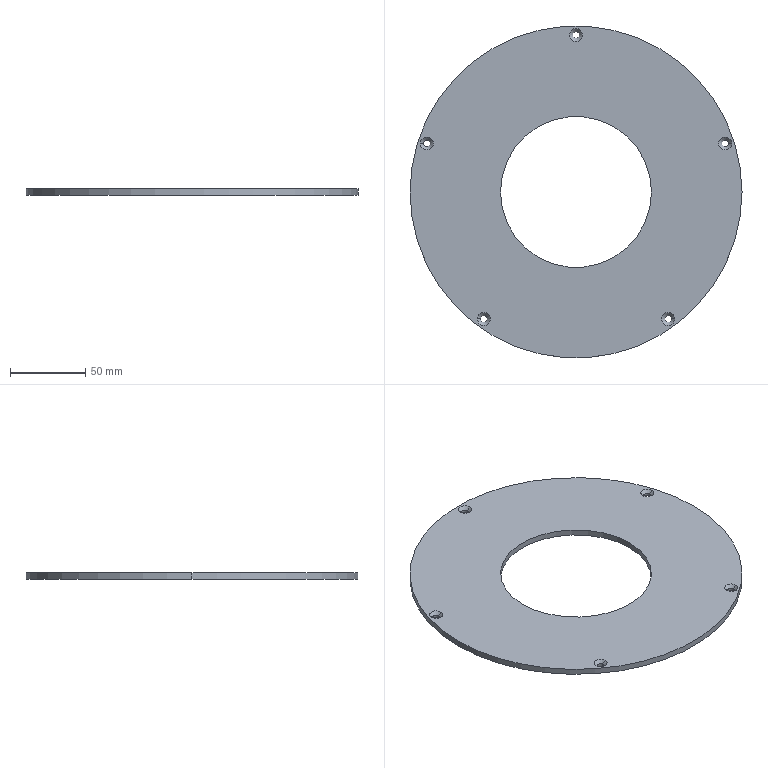Part | SolidWorks | features Extrusion 1, HoleWzd 1 | 1 solid | 26 faces | box 220 x 220 x 4 mm | volume 120125 mm3 | cylinder 14 | cone 10 | plane 2 | commonest cylinder face diameters 4.5 x10 100 x2 220 x2
STEP:
#1=CARTESIAN_POINT('',(-2.25,104.,1.95));
#2=VERTEX_POINT('',#1);
#3=CARTESIAN_POINT('',(2.25,104.,1.95));
#4=VERTEX_POINT('',#3);
#5=CARTESIAN_POINT('',(0.,104.,1.95));
#6=DIRECTION('',(0.,0.,1.));
#7=DIRECTION('',(1.,0.,0.));
#8=AXIS2_PLACEMENT_3D('',#5,#6,#7);
#9=CIRCLE('',#8,2.25);
#10=EDGE_CURVE('',#2,#4,#9,.T.);
#11=ORIENTED_EDGE('',*,*,#10,.F.);
#12=CARTESIAN_POINT('',(-4.3,104.,4.));
#13=VERTEX_POINT('',#12);
#14=CARTESIAN_POINT('',(-4.3,104.,4.));
#15=DIRECTION('',(-0.7071,0.,0.7071));
#16=VECTOR('',#15,1000.);
#17=LINE('',#14,#16);
#18=EDGE_CURVE('',#2,#13,#17,.T.);
#19=ORIENTED_EDGE('',*,*,#18,.T.);
#20=CARTESIAN_POINT('',(4.3,104.,4.));
#21=VERTEX_POINT('',#20);
#22=CARTESIAN_POINT('',(0.,104.,4.));
#23=DIRECTION('',(0.,0.,1.));
#24=DIRECTION('',(1.,0.,0.));
#25=AXIS2_PLACEMENT_3D('',#22,#23,#24);
#26=CIRCLE('',#25,4.3);
#27=EDGE_CURVE('',#13,#21,#26,.T.);
#28=ORIENTED_EDGE('',*,*,#27,.T.);
#29=CARTESIAN_POINT('',(4.3,104.,4.));
#30=DIRECTION('',(0.7071,0.,0.7071));
#31=VECTOR('',#30,1000.);
#32=LINE('',#29,#31);
#33=EDGE_CURVE('',#4,#21,#32,.T.);
#34=ORIENTED_EDGE('',*,*,#33,.F.);
#35=EDGE_LOOP('',(#11,#19,#28,#34));
#36=FACE_OUTER_BOUND('',#35,.T.);
#37=CARTESIAN_POINT('',(0.,104.,4.));
#38=DIRECTION('',(0.,0.,1.));
#39=DIRECTION('',(1.,0.,0.));
#40=AXIS2_PLACEMENT_3D('',#37,#38,#39);
#41=CONICAL_SURFACE('',#40,4.3,0.7854);
#42=ADVANCED_FACE('',(#36),#41,.F.);
#43=CARTESIAN_POINT('',(-2.25,104.,0.));
#44=VERTEX_POINT('',#43);
#45=CARTESIAN_POINT('',(2.25,104.,0.));
#46=VERTEX_POINT('',#45);
#47=CARTESIAN_POINT('',(0.,104.,0.));
#48=DIRECTION('',(0.,0.,1.));
#49=DIRECTION('',(1.,0.,0.));
#50=AXIS2_PLACEMENT_3D('',#47,#48,#49);
#51=CIRCLE('',#50,2.25);
#52=EDGE_CURVE('',#44,#46,#51,.T.);
#53=ORIENTED_EDGE('',*,*,#52,.F.);
#54=CARTESIAN_POINT('',(-2.25,104.,4.));
#55=DIRECTION('',(0.,0.,1.));
#56=VECTOR('',#55,1000.);
#57=LINE('',#54,#56);
#58=EDGE_CURVE('',#44,#2,#57,.T.);
#59=ORIENTED_EDGE('',*,*,#58,.T.);
#60=ORIENTED_EDGE('',*,*,#10,.T.);
#61=CARTESIAN_POINT('',(2.25,104.,4.));
#62=DIRECTION('',(0.,0.,1.));
#63=VECTOR('',#62,1000.);
#64=LINE('',#61,#63);
#65=EDGE_CURVE('',#46,#4,#64,.T.);
#66=ORIENTED_EDGE('',*,*,#65,.F.);
#67=EDGE_LOOP('',(#53,#59,#60,#66));
#68=FACE_OUTER_BOUND('',#67,.T.);
#69=CARTESIAN_POINT('',(0.,104.,4.));
#70=DIRECTION('',(0.,0.,1.));
#71=DIRECTION('',(1.,0.,0.));
#72=AXIS2_PLACEMENT_3D('',#69,#70,#71);
#73=CYLINDRICAL_SURFACE('',#72,2.25);
#74=ADVANCED_FACE('',(#68),#73,.F.);
#75=CARTESIAN_POINT('',(96.66,32.138,1.95));
#76=VERTEX_POINT('',#75);
#77=CARTESIAN_POINT('',(101.16,32.138,1.95));
#78=VERTEX_POINT('',#77);
#79=CARTESIAN_POINT('',(98.91,32.138,1.95));
#80=DIRECTION('',(0.,0.,1.));
#81=DIRECTION('',(1.,0.,0.));
#82=AXIS2_PLACEMENT_3D('',#79,#80,#81);
#83=CIRCLE('',#82,2.25);
#84=EDGE_CURVE('',#76,#78,#83,.T.);
#85=ORIENTED_EDGE('',*,*,#84,.F.);
#86=CARTESIAN_POINT('',(94.61,32.138,4.));
#87=VERTEX_POINT('',#86);
#88=CARTESIAN_POINT('',(94.61,32.138,4.));
#89=DIRECTION('',(-0.7071,0.,0.7071));
#90=VECTOR('',#89,1000.);
#91=LINE('',#88,#90);
#92=EDGE_CURVE('',#76,#87,#91,.T.);
#93=ORIENTED_EDGE('',*,*,#92,.T.);
#94=CARTESIAN_POINT('',(103.21,32.138,4.));
#95=VERTEX_POINT('',#94);
#96=CARTESIAN_POINT('',(98.91,32.138,4.));
#97=DIRECTION('',(0.,0.,1.));
#98=DIRECTION('',(1.,0.,0.));
#99=AXIS2_PLACEMENT_3D('',#96,#97,#98);
#100=CIRCLE('',#99,4.3);
#101=EDGE_CURVE('',#87,#95,#100,.T.);
#102=ORIENTED_EDGE('',*,*,#101,.T.);
#103=CARTESIAN_POINT('',(103.21,32.138,4.));
#104=DIRECTION('',(0.7071,0.,0.7071));
#105=VECTOR('',#104,1000.);
#106=LINE('',#103,#105);
#107=EDGE_CURVE('',#78,#95,#106,.T.);
#108=ORIENTED_EDGE('',*,*,#107,.F.);
#109=EDGE_LOOP('',(#85,#93,#102,#108));
#110=FACE_OUTER_BOUND('',#109,.T.);
#111=CARTESIAN_POINT('',(98.91,32.138,4.));
#112=DIRECTION('',(0.,0.,1.));
#113=DIRECTION('',(1.,0.,0.));
#114=AXIS2_PLACEMENT_3D('',#111,#112,#113);
#115=CONICAL_SURFACE('',#114,4.3,0.7854);
#116=ADVANCED_FACE('',(#110),#115,.F.);
#117=CARTESIAN_POINT('',(96.66,32.138,0.));
#118=VERTEX_POINT('',#117);
#119=CARTESIAN_POINT('',(101.16,32.138,0.));
#120=VERTEX_POINT('',#119);
#121=CARTESIAN_POINT('',(98.91,32.138,0.));
#122=DIRECTION('',(0.,0.,1.));
#123=DIRECTION('',(1.,0.,0.));
#124=AXIS2_PLACEMENT_3D('',#121,#122,#123);
#125=CIRCLE('',#124,2.25);
#126=EDGE_CURVE('',#118,#120,#125,.T.);
#127=ORIENTED_EDGE('',*,*,#126,.F.);
#128=CARTESIAN_POINT('',(96.66,32.138,4.));
#129=DIRECTION('',(0.,0.,1.));
#130=VECTOR('',#129,1000.);
#131=LINE('',#128,#130);
#132=EDGE_CURVE('',#118,#76,#131,.T.);
#133=ORIENTED_EDGE('',*,*,#132,.T.);
#134=ORIENTED_EDGE('',*,*,#84,.T.);
#135=CARTESIAN_POINT('',(101.16,32.138,4.));
#136=DIRECTION('',(0.,0.,1.));
#137=VECTOR('',#136,1000.);
#138=LINE('',#135,#137);
#139=EDGE_CURVE('',#120,#78,#138,.T.);
#140=ORIENTED_EDGE('',*,*,#139,.F.);
#141=EDGE_LOOP('',(#127,#133,#134,#140));
#142=FACE_OUTER_BOUND('',#141,.T.);
#143=CARTESIAN_POINT('',(98.91,32.138,4.));
#144=DIRECTION('',(0.,0.,1.));
#145=DIRECTION('',(1.,0.,0.));
#146=AXIS2_PLACEMENT_3D('',#143,#144,#145);
#147=CYLINDRICAL_SURFACE('',#146,2.25);
#148=ADVANCED_FACE('',(#142),#147,.F.);
#149=CARTESIAN_POINT('',(58.88,-84.138,1.95));
#150=VERTEX_POINT('',#149);
#151=CARTESIAN_POINT('',(63.38,-84.138,1.95));
#152=VERTEX_POINT('',#151);
#153=CARTESIAN_POINT('',(61.13,-84.138,1.95));
#154=DIRECTION('',(0.,0.,1.));
#155=DIRECTION('',(1.,0.,0.));
#156=AXIS2_PLACEMENT_3D('',#153,#154,#155);
#157=CIRCLE('',#156,2.25);
#158=EDGE_CURVE('',#150,#152,#157,.T.);
#159=ORIENTED_EDGE('',*,*,#158,.F.);
#160=CARTESIAN_POINT('',(56.83,-84.138,4.));
#161=VERTEX_POINT('',#160);
#162=CARTESIAN_POINT('',(56.83,-84.138,4.));
#163=DIRECTION('',(-0.7071,0.,0.7071));
#164=VECTOR('',#163,1000.);
#165=LINE('',#162,#164);
#166=EDGE_CURVE('',#150,#161,#165,.T.);
#167=ORIENTED_EDGE('',*,*,#166,.T.);
#168=CARTESIAN_POINT('',(65.43,-84.138,4.));
#169=VERTEX_POINT('',#168);
#170=CARTESIAN_POINT('',(61.13,-84.138,4.));
#171=DIRECTION('',(0.,0.,1.));
#172=DIRECTION('',(1.,0.,0.));
#173=AXIS2_PLACEMENT_3D('',#170,#171,#172);
#174=CIRCLE('',#173,4.3);
#175=EDGE_CURVE('',#161,#169,#174,.T.);
#176=ORIENTED_EDGE('',*,*,#175,.T.);
#177=CARTESIAN_POINT('',(65.43,-84.138,4.));
#178=DIRECTION('',(0.7071,0.,0.7071));
#179=VECTOR('',#178,1000.);
#180=LINE('',#177,#179);
#181=EDGE_CURVE('',#152,#169,#180,.T.);
#182=ORIENTED_EDGE('',*,*,#181,.F.);
#183=EDGE_LOOP('',(#159,#167,#176,#182));
#184=FACE_OUTER_BOUND('',#183,.T.);
#185=CARTESIAN_POINT('',(61.13,-84.138,4.));
#186=DIRECTION('',(0.,0.,1.));
#187=DIRECTION('',(1.,0.,0.));
#188=AXIS2_PLACEMENT_3D('',#185,#186,#187);
#189=CONICAL_SURFACE('',#188,4.3,0.7854);
#190=ADVANCED_FACE('',(#184),#189,.F.);
#191=CARTESIAN_POINT('',(58.88,-84.138,0.));
#192=VERTEX_POINT('',#191);
#193=CARTESIAN_POINT('',(63.38,-84.138,0.));
#194=VERTEX_POINT('',#193);
#195=CARTESIAN_POINT('',(61.13,-84.138,0.));
#196=DIRECTION('',(0.,0.,1.));
#197=DIRECTION('',(1.,0.,0.));
#198=AXIS2_PLACEMENT_3D('',#195,#196,#197);
#199=CIRCLE('',#198,2.25);
#200=EDGE_CURVE('',#192,#194,#199,.T.);
#201=ORIENTED_EDGE('',*,*,#200,.F.);
#202=CARTESIAN_POINT('',(58.88,-84.138,4.));
#203=DIRECTION('',(0.,0.,1.));
#204=VECTOR('',#203,1000.);
#205=LINE('',#202,#204);
#206=EDGE_CURVE('',#192,#150,#205,.T.);
#207=ORIENTED_EDGE('',*,*,#206,.T.);
#208=ORIENTED_EDGE('',*,*,#158,.T.);
#209=CARTESIAN_POINT('',(63.38,-84.138,4.));
#210=DIRECTION('',(0.,0.,1.));
#211=VECTOR('',#210,1000.);
#212=LINE('',#209,#211);
#213=EDGE_CURVE('',#194,#152,#212,.T.);
#214=ORIENTED_EDGE('',*,*,#213,.F.);
#215=EDGE_LOOP('',(#201,#207,#208,#214));
#216=FACE_OUTER_BOUND('',#215,.T.);
#217=CARTESIAN_POINT('',(61.13,-84.138,4.));
#218=DIRECTION('',(0.,0.,1.));
#219=DIRECTION('',(1.,0.,0.));
#220=AXIS2_PLACEMENT_3D('',#217,#218,#219);
#221=CYLINDRICAL_SURFACE('',#220,2.25);
#222=ADVANCED_FACE('',(#216),#221,.F.);
#223=CARTESIAN_POINT('',(-63.38,-84.138,1.95));
#224=VERTEX_POINT('',#223);
#225=CARTESIAN_POINT('',(-58.88,-84.138,1.95));
#226=VERTEX_POINT('',#225);
#227=CARTESIAN_POINT('',(-61.13,-84.138,1.95));
#228=DIRECTION('',(0.,0.,1.));
#229=DIRECTION('',(1.,0.,0.));
#230=AXIS2_PLACEMENT_3D('',#227,#228,#229);
#231=CIRCLE('',#230,2.25);
#232=EDGE_CURVE('',#224,#226,#231,.T.);
#233=ORIENTED_EDGE('',*,*,#232,.F.);
#234=CARTESIAN_POINT('',(-65.43,-84.138,4.));
#235=VERTEX_POINT('',#234);
#236=CARTESIAN_POINT('',(-65.43,-84.138,4.));
#237=DIRECTION('',(-0.7071,0.,0.7071));
#238=VECTOR('',#237,1000.);
#239=LINE('',#236,#238);
#240=EDGE_CURVE('',#224,#235,#239,.T.);
#241=ORIENTED_EDGE('',*,*,#240,.T.);
#242=CARTESIAN_POINT('',(-56.83,-84.138,4.));
#243=VERTEX_POINT('',#242);
#244=CARTESIAN_POINT('',(-61.13,-84.138,4.));
#245=DIRECTION('',(0.,0.,1.));
#246=DIRECTION('',(1.,0.,0.));
#247=AXIS2_PLACEMENT_3D('',#244,#245,#246);
#248=CIRCLE('',#247,4.3);
#249=EDGE_CURVE('',#235,#243,#248,.T.);
#250=ORIENTED_EDGE('',*,*,#249,.T.);
#251=CARTESIAN_POINT('',(-56.83,-84.138,4.));
#252=DIRECTION('',(0.7071,0.,0.7071));
#253=VECTOR('',#252,1000.);
#254=LINE('',#251,#253);
#255=EDGE_CURVE('',#226,#243,#254,.T.);
#256=ORIENTED_EDGE('',*,*,#255,.F.);
#257=EDGE_LOOP('',(#233,#241,#250,#256));
#258=FACE_OUTER_BOUND('',#257,.T.);
#259=CARTESIAN_POINT('',(-61.13,-84.138,4.));
#260=DIRECTION('',(0.,0.,1.));
#261=DIRECTION('',(1.,0.,0.));
#262=AXIS2_PLACEMENT_3D('',#259,#260,#261);
#263=CONICAL_SURFACE('',#262,4.3,0.7854);
#264=ADVANCED_FACE('',(#258),#263,.F.);
#265=CARTESIAN_POINT('',(-63.38,-84.138,0.));
#266=VERTEX_POINT('',#265);
#267=CARTESIAN_POINT('',(-58.88,-84.138,0.));
#268=VERTEX_POINT('',#267);
#269=CARTESIAN_POINT('',(-61.13,-84.138,0.));
#270=DIRECTION('',(0.,0.,1.));
#271=DIRECTION('',(1.,0.,0.));
#272=AXIS2_PLACEMENT_3D('',#269,#270,#271);
#273=CIRCLE('',#272,2.25);
#274=EDGE_CURVE('',#266,#268,#273,.T.);
#275=ORIENTED_EDGE('',*,*,#274,.F.);
#276=CARTESIAN_POINT('',(-63.38,-84.138,4.));
#277=DIRECTION('',(0.,0.,1.));
#278=VECTOR('',#277,1000.);
#279=LINE('',#276,#278);
#280=EDGE_CURVE('',#266,#224,#279,.T.);
#281=ORIENTED_EDGE('',*,*,#280,.T.);
#282=ORIENTED_EDGE('',*,*,#232,.T.);
#283=CARTESIAN_POINT('',(-58.88,-84.138,4.));
#284=DIRECTION('',(0.,0.,1.));
#285=VECTOR('',#284,1000.);
#286=LINE('',#283,#285);
#287=EDGE_CURVE('',#268,#226,#286,.T.);
#288=ORIENTED_EDGE('',*,*,#287,.F.);
#289=EDGE_LOOP('',(#275,#281,#282,#288));
#290=FACE_OUTER_BOUND('',#289,.T.);
#291=CARTESIAN_POINT('',(-61.13,-84.138,4.));
#292=DIRECTION('',(0.,0.,1.));
#293=DIRECTION('',(1.,0.,0.));
#294=AXIS2_PLACEMENT_3D('',#291,#292,#293);
#295=CYLINDRICAL_SURFACE('',#294,2.25);
#296=ADVANCED_FACE('',(#290),#295,.F.);
#297=CARTESIAN_POINT('',(-101.16,32.138,1.95));
#298=VERTEX_POINT('',#297);
#299=CARTESIAN_POINT('',(-96.66,32.138,1.95));
#300=VERTEX_POINT('',#299);
#301=CARTESIAN_POINT('',(-98.91,32.138,1.95));
#302=DIRECTION('',(0.,0.,1.));
#303=DIRECTION('',(1.,0.,0.));
#304=AXIS2_PLACEMENT_3D('',#301,#302,#303);
#305=CIRCLE('',#304,2.25);
#306=EDGE_CURVE('',#298,#300,#305,.T.);
#307=ORIENTED_EDGE('',*,*,#306,.F.);
#308=CARTESIAN_POINT('',(-103.21,32.138,4.));
#309=VERTEX_POINT('',#308);
#310=CARTESIAN_POINT('',(-103.21,32.138,4.));
#311=DIRECTION('',(-0.7071,0.,0.7071));
#312=VECTOR('',#311,1000.);
#313=LINE('',#310,#312);
#314=EDGE_CURVE('',#298,#309,#313,.T.);
#315=ORIENTED_EDGE('',*,*,#314,.T.);
#316=CARTESIAN_POINT('',(-94.61,32.138,4.));
#317=VERTEX_POINT('',#316);
#318=CARTESIAN_POINT('',(-98.91,32.138,4.));
#319=DIRECTION('',(0.,0.,1.));
#320=DIRECTION('',(1.,0.,0.));
#321=AXIS2_PLACEMENT_3D('',#318,#319,#320);
#322=CIRCLE('',#321,4.3);
#323=EDGE_CURVE('',#309,#317,#322,.T.);
#324=ORIENTED_EDGE('',*,*,#323,.T.);
#325=CARTESIAN_POINT('',(-94.61,32.138,4.));
#326=DIRECTION('',(0.7071,0.,0.7071));
#327=VECTOR('',#326,1000.);
#328=LINE('',#325,#327);
#329=EDGE_CURVE('',#300,#317,#328,.T.);
#330=ORIENTED_EDGE('',*,*,#329,.F.);
#331=EDGE_LOOP('',(#307,#315,#324,#330));
#332=FACE_OUTER_BOUND('',#331,.T.);
#333=CARTESIAN_POINT('',(-98.91,32.138,4.));
#334=DIRECTION('',(0.,0.,1.));
#335=DIRECTION('',(1.,0.,0.));
#336=AXIS2_PLACEMENT_3D('',#333,#334,#335);
#337=CONICAL_SURFACE('',#336,4.3,0.7854);
#338=ADVANCED_FACE('',(#332),#337,.F.);
#339=CARTESIAN_POINT('',(-101.16,32.138,0.));
#340=VERTEX_POINT('',#339);
#341=CARTESIAN_POINT('',(-96.66,32.138,0.));
#342=VERTEX_POINT('',#341);
#343=CARTESIAN_POINT('',(-98.91,32.138,0.));
#344=DIRECTION('',(0.,0.,1.));
#345=DIRECTION('',(1.,0.,0.));
#346=AXIS2_PLACEMENT_3D('',#343,#344,#345);
#347=CIRCLE('',#346,2.25);
#348=EDGE_CURVE('',#340,#342,#347,.T.);
#349=ORIENTED_EDGE('',*,*,#348,.F.);
#350=CARTESIAN_POINT('',(-101.16,32.138,4.));
#351=DIRECTION('',(0.,0.,1.));
#352=VECTOR('',#351,1000.);
#353=LINE('',#350,#352);
#354=EDGE_CURVE('',#340,#298,#353,.T.);
#355=ORIENTED_EDGE('',*,*,#354,.T.);
#356=ORIENTED_EDGE('',*,*,#306,.T.);
#357=CARTESIAN_POINT('',(-96.66,32.138,4.));
#358=DIRECTION('',(0.,0.,1.));
#359=VECTOR('',#358,1000.);
#360=LINE('',#357,#359);
#361=EDGE_CURVE('',#342,#300,#360,.T.);
#362=ORIENTED_EDGE('',*,*,#361,.F.);
#363=EDGE_LOOP('',(#349,#355,#356,#362));
#364=FACE_OUTER_BOUND('',#363,.T.);
#365=CARTESIAN_POINT('',(-98.91,32.138,4.));
#366=DIRECTION('',(0.,0.,1.));
#367=DIRECTION('',(1.,0.,0.));
#368=AXIS2_PLACEMENT_3D('',#365,#366,#367);
#369=CYLINDRICAL_SURFACE('',#368,2.25);
#370=ADVANCED_FACE('',(#364),#369,.F.);
#371=CARTESIAN_POINT('',(-50.,0.,4.));
#372=VERTEX_POINT('',#371);
#373=CARTESIAN_POINT('',(50.,0.,4.));
#374=VERTEX_POINT('',#373);
#375=CARTESIAN_POINT('',(0.,0.,4.));
#376=DIRECTION('',(0.,0.,1.));
#377=DIRECTION('',(1.,0.,0.));
#378=AXIS2_PLACEMENT_3D('',#375,#376,#377);
#379=CIRCLE('',#378,50.);
#380=EDGE_CURVE('',#372,#374,#379,.T.);
#381=ORIENTED_EDGE('',*,*,#380,.T.);
#382=CARTESIAN_POINT('',(50.,0.,0.));
#383=VERTEX_POINT('',#382);
#384=CARTESIAN_POINT('',(50.,0.,4.));
#385=DIRECTION('',(0.,0.,-1.));
#386=VECTOR('',#385,1000.);
#387=LINE('',#384,#386);
#388=EDGE_CURVE('',#374,#383,#387,.T.);
#389=ORIENTED_EDGE('',*,*,#388,.T.);
#390=CARTESIAN_POINT('',(-50.,0.,0.));
#391=VERTEX_POINT('',#390);
#392=CARTESIAN_POINT('',(0.,0.,0.));
#393=DIRECTION('',(0.,0.,1.));
#394=DIRECTION('',(1.,0.,0.));
#395=AXIS2_PLACEMENT_3D('',#392,#393,#394);
#396=CIRCLE('',#395,50.);
#397=EDGE_CURVE('',#391,#383,#396,.T.);
#398=ORIENTED_EDGE('',*,*,#397,.F.);
#399=CARTESIAN_POINT('',(-50.,0.,4.));
#400=DIRECTION('',(0.,0.,-1.));
#401=VECTOR('',#400,1000.);
#402=LINE('',#399,#401);
#403=EDGE_CURVE('',#372,#391,#402,.T.);
#404=ORIENTED_EDGE('',*,*,#403,.F.);
#405=EDGE_LOOP('',(#381,#389,#398,#404));
#406=FACE_OUTER_BOUND('',#405,.T.);
#407=CARTESIAN_POINT('',(0.,0.,4.));
#408=DIRECTION('',(0.,0.,-1.));
#409=DIRECTION('',(-1.,0.,0.));
#410=AXIS2_PLACEMENT_3D('',#407,#408,#409);
#411=CYLINDRICAL_SURFACE('',#410,50.);
#412=ADVANCED_FACE('',(#406),#411,.F.);
#413=CARTESIAN_POINT('',(110.,0.,4.));
#414=VERTEX_POINT('',#413);
#415=CARTESIAN_POINT('',(-110.,0.,4.));
#416=VERTEX_POINT('',#415);
#417=CARTESIAN_POINT('',(0.,0.,4.));
#418=DIRECTION('',(0.,0.,1.));
#419=DIRECTION('',(1.,0.,0.));
#420=AXIS2_PLACEMENT_3D('',#417,#418,#419);
#421=CIRCLE('',#420,110.);
#422=EDGE_CURVE('',#414,#416,#421,.T.);
#423=ORIENTED_EDGE('',*,*,#422,.F.);
#424=CARTESIAN_POINT('',(110.,0.,0.));
#425=VERTEX_POINT('',#424);
#426=CARTESIAN_POINT('',(110.,0.,4.));
#427=DIRECTION('',(0.,0.,-1.));
#428=VECTOR('',#427,1000.);
#429=LINE('',#426,#428);
#430=EDGE_CURVE('',#414,#425,#429,.T.);
#431=ORIENTED_EDGE('',*,*,#430,.T.);
#432=CARTESIAN_POINT('',(-110.,0.,0.));
#433=VERTEX_POINT('',#432);
#434=CARTESIAN_POINT('',(0.,0.,0.));
#435=DIRECTION('',(0.,0.,1.));
#436=DIRECTION('',(1.,0.,0.));
#437=AXIS2_PLACEMENT_3D('',#434,#435,#436);
#438=CIRCLE('',#437,110.);
#439=EDGE_CURVE('',#425,#433,#438,.T.);
#440=ORIENTED_EDGE('',*,*,#439,.T.);
#441=CARTESIAN_POINT('',(-110.,0.,4.));
#442=DIRECTION('',(0.,0.,-1.));
#443=VECTOR('',#442,1000.);
#444=LINE('',#441,#443);
#445=EDGE_CURVE('',#416,#433,#444,.T.);
#446=ORIENTED_EDGE('',*,*,#445,.F.);
#447=EDGE_LOOP('',(#423,#431,#440,#446));
#448=FACE_OUTER_BOUND('',#447,.T.);
#449=CARTESIAN_POINT('',(0.,0.,4.));
#450=DIRECTION('',(0.,0.,-1.));
#451=DIRECTION('',(-1.,0.,0.));
#452=AXIS2_PLACEMENT_3D('',#449,#450,#451);
#453=CYLINDRICAL_SURFACE('',#452,110.);
#454=ADVANCED_FACE('',(#448),#453,.T.);
#455=CARTESIAN_POINT('',(0.,104.,4.));
#456=DIRECTION('',(0.,0.,1.));
#457=DIRECTION('',(1.,0.,0.));
#458=AXIS2_PLACEMENT_3D('',#455,#456,#457);
#459=CIRCLE('',#458,4.3);
#460=EDGE_CURVE('',#21,#13,#459,.T.);
#461=ORIENTED_EDGE('',*,*,#460,.F.);
#462=ORIENTED_EDGE('',*,*,#27,.F.);
#463=EDGE_LOOP('',(#461,#462));
#464=FACE_BOUND('',#463,.T.);
#465=CARTESIAN_POINT('',(98.91,32.138,4.));
#466=DIRECTION('',(0.,0.,1.));
#467=DIRECTION('',(1.,0.,0.));
#468=AXIS2_PLACEMENT_3D('',#465,#466,#467);
#469=CIRCLE('',#468,4.3);
#470=EDGE_CURVE('',#95,#87,#469,.T.);
#471=ORIENTED_EDGE('',*,*,#470,.F.);
#472=ORIENTED_EDGE('',*,*,#101,.F.);
#473=EDGE_LOOP('',(#471,#472));
#474=FACE_BOUND('',#473,.T.);
#475=CARTESIAN_POINT('',(61.13,-84.138,4.));
#476=DIRECTION('',(0.,0.,1.));
#477=DIRECTION('',(1.,0.,0.));
#478=AXIS2_PLACEMENT_3D('',#475,#476,#477);
#479=CIRCLE('',#478,4.3);
#480=EDGE_CURVE('',#169,#161,#479,.T.);
#481=ORIENTED_EDGE('',*,*,#480,.F.);
#482=ORIENTED_EDGE('',*,*,#175,.F.);
#483=EDGE_LOOP('',(#481,#482));
#484=FACE_BOUND('',#483,.T.);
#485=CARTESIAN_POINT('',(-61.13,-84.138,4.));
#486=DIRECTION('',(0.,0.,1.));
#487=DIRECTION('',(1.,0.,0.));
#488=AXIS2_PLACEMENT_3D('',#485,#486,#487);
#489=CIRCLE('',#488,4.3);
#490=EDGE_CURVE('',#243,#235,#489,.T.);
#491=ORIENTED_EDGE('',*,*,#490,.F.);
#492=ORIENTED_EDGE('',*,*,#249,.F.);
#493=EDGE_LOOP('',(#491,#492));
#494=FACE_BOUND('',#493,.T.);
#495=CARTESIAN_POINT('',(-98.91,32.138,4.));
#496=DIRECTION('',(0.,0.,1.));
#497=DIRECTION('',(1.,0.,0.));
#498=AXIS2_PLACEMENT_3D('',#495,#496,#497);
#499=CIRCLE('',#498,4.3);
#500=EDGE_CURVE('',#317,#309,#499,.T.);
#501=ORIENTED_EDGE('',*,*,#500,.F.);
#502=ORIENTED_EDGE('',*,*,#323,.F.);
#503=EDGE_LOOP('',(#501,#502));
#504=FACE_BOUND('',#503,.T.);
#505=CARTESIAN_POINT('',(0.,0.,4.));
#506=DIRECTION('',(0.,0.,1.));
#507=DIRECTION('',(1.,0.,0.));
#508=AXIS2_PLACEMENT_3D('',#505,#506,#507);
#509=CIRCLE('',#508,110.);
#510=EDGE_CURVE('',#416,#414,#509,.T.);
#511=ORIENTED_EDGE('',*,*,#510,.T.);
#512=ORIENTED_EDGE('',*,*,#422,.T.);
#513=EDGE_LOOP('',(#511,#512));
#514=FACE_OUTER_BOUND('',#513,.T.);
#515=ORIENTED_EDGE('',*,*,#380,.F.);
#516=CARTESIAN_POINT('',(0.,0.,4.));
#517=DIRECTION('',(0.,0.,1.));
#518=DIRECTION('',(1.,0.,0.));
#519=AXIS2_PLACEMENT_3D('',#516,#517,#518);
#520=CIRCLE('',#519,50.);
#521=EDGE_CURVE('',#374,#372,#520,.T.);
#522=ORIENTED_EDGE('',*,*,#521,.F.);
#523=EDGE_LOOP('',(#515,#522));
#524=FACE_BOUND('',#523,.T.);
#525=CARTESIAN_POINT('',(0.,0.,4.));
#526=DIRECTION('',(0.,0.,1.));
#527=DIRECTION('',(1.,0.,0.));
#528=AXIS2_PLACEMENT_3D('',#525,#526,#527);
#529=PLANE('',#528);
#530=ADVANCED_FACE('',(#464,#474,#484,#494,#504,#514,#524),#529,.T.);
#531=CARTESIAN_POINT('',(0.,104.,0.));
#532=DIRECTION('',(0.,0.,1.));
#533=DIRECTION('',(1.,0.,0.));
#534=AXIS2_PLACEMENT_3D('',#531,#532,#533);
#535=CIRCLE('',#534,2.25);
#536=EDGE_CURVE('',#46,#44,#535,.T.);
#537=ORIENTED_EDGE('',*,*,#536,.T.);
#538=ORIENTED_EDGE('',*,*,#52,.T.);
#539=EDGE_LOOP('',(#537,#538));
#540=FACE_BOUND('',#539,.T.);
#541=CARTESIAN_POINT('',(98.91,32.138,0.));
#542=DIRECTION('',(0.,0.,1.));
#543=DIRECTION('',(1.,0.,0.));
#544=AXIS2_PLACEMENT_3D('',#541,#542,#543);
#545=CIRCLE('',#544,2.25);
#546=EDGE_CURVE('',#120,#118,#545,.T.);
#547=ORIENTED_EDGE('',*,*,#546,.T.);
#548=ORIENTED_EDGE('',*,*,#126,.T.);
#549=EDGE_LOOP('',(#547,#548));
#550=FACE_BOUND('',#549,.T.);
#551=CARTESIAN_POINT('',(61.13,-84.138,0.));
#552=DIRECTION('',(0.,0.,1.));
#553=DIRECTION('',(1.,0.,0.));
#554=AXIS2_PLACEMENT_3D('',#551,#552,#553);
#555=CIRCLE('',#554,2.25);
#556=EDGE_CURVE('',#194,#192,#555,.T.);
#557=ORIENTED_EDGE('',*,*,#556,.T.);
#558=ORIENTED_EDGE('',*,*,#200,.T.);
#559=EDGE_LOOP('',(#557,#558));
#560=FACE_BOUND('',#559,.T.);
#561=CARTESIAN_POINT('',(-61.13,-84.138,0.));
#562=DIRECTION('',(0.,0.,1.));
#563=DIRECTION('',(1.,0.,0.));
#564=AXIS2_PLACEMENT_3D('',#561,#562,#563);
#565=CIRCLE('',#564,2.25);
#566=EDGE_CURVE('',#268,#266,#565,.T.);
#567=ORIENTED_EDGE('',*,*,#566,.T.);
#568=ORIENTED_EDGE('',*,*,#274,.T.);
#569=EDGE_LOOP('',(#567,#568));
#570=FACE_BOUND('',#569,.T.);
#571=CARTESIAN_POINT('',(-98.91,32.138,0.));
#572=DIRECTION('',(0.,0.,1.));
#573=DIRECTION('',(1.,0.,0.));
#574=AXIS2_PLACEMENT_3D('',#571,#572,#573);
#575=CIRCLE('',#574,2.25);
#576=EDGE_CURVE('',#342,#340,#575,.T.);
#577=ORIENTED_EDGE('',*,*,#576,.T.);
#578=ORIENTED_EDGE('',*,*,#348,.T.);
#579=EDGE_LOOP('',(#577,#578));
#580=FACE_BOUND('',#579,.T.);
#581=CARTESIAN_POINT('',(0.,0.,0.));
#582=DIRECTION('',(0.,0.,1.));
#583=DIRECTION('',(1.,0.,0.));
#584=AXIS2_PLACEMENT_3D('',#581,#582,#583);
#585=CIRCLE('',#584,110.);
#586=EDGE_CURVE('',#433,#425,#585,.T.);
#587=ORIENTED_EDGE('',*,*,#586,.F.);
#588=ORIENTED_EDGE('',*,*,#439,.F.);
#589=EDGE_LOOP('',(#587,#588));
#590=FACE_OUTER_BOUND('',#589,.T.);
#591=ORIENTED_EDGE('',*,*,#397,.T.);
#592=CARTESIAN_POINT('',(0.,0.,0.));
#593=DIRECTION('',(0.,0.,1.));
#594=DIRECTION('',(1.,0.,0.));
#595=AXIS2_PLACEMENT_3D('',#592,#593,#594);
#596=CIRCLE('',#595,50.);
#597=EDGE_CURVE('',#383,#391,#596,.T.);
#598=ORIENTED_EDGE('',*,*,#597,.T.);
#599=EDGE_LOOP('',(#591,#598));
#600=FACE_BOUND('',#599,.T.);
#601=CARTESIAN_POINT('',(0.,0.,0.));
#602=DIRECTION('',(0.,0.,1.));
#603=DIRECTION('',(1.,0.,0.));
#604=AXIS2_PLACEMENT_3D('',#601,#602,#603);
#605=PLANE('',#604);
#606=ADVANCED_FACE('',(#540,#550,#560,#570,#580,#590,#600),#605,.F.);
#607=ORIENTED_EDGE('',*,*,#430,.F.);
#608=ORIENTED_EDGE('',*,*,#510,.F.);
#609=ORIENTED_EDGE('',*,*,#445,.T.);
#610=ORIENTED_EDGE('',*,*,#586,.T.);
#611=EDGE_LOOP('',(#607,#608,#609,#610));
#612=FACE_OUTER_BOUND('',#611,.T.);
#613=CARTESIAN_POINT('',(0.,0.,4.));
#614=DIRECTION('',(0.,0.,-1.));
#615=DIRECTION('',(-1.,0.,0.));
#616=AXIS2_PLACEMENT_3D('',#613,#614,#615);
#617=CYLINDRICAL_SURFACE('',#616,110.);
#618=ADVANCED_FACE('',(#612),#617,.T.);
#619=ORIENTED_EDGE('',*,*,#388,.F.);
#620=ORIENTED_EDGE('',*,*,#521,.T.);
#621=ORIENTED_EDGE('',*,*,#403,.T.);
#622=ORIENTED_EDGE('',*,*,#597,.F.);
#623=EDGE_LOOP('',(#619,#620,#621,#622));
#624=FACE_OUTER_BOUND('',#623,.T.);
#625=CARTESIAN_POINT('',(0.,0.,4.));
#626=DIRECTION('',(0.,0.,-1.));
#627=DIRECTION('',(-1.,0.,0.));
#628=AXIS2_PLACEMENT_3D('',#625,#626,#627);
#629=CYLINDRICAL_SURFACE('',#628,50.);
#630=ADVANCED_FACE('',(#624),#629,.F.);
#631=ORIENTED_EDGE('',*,*,#354,.F.);
#632=ORIENTED_EDGE('',*,*,#576,.F.);
#633=ORIENTED_EDGE('',*,*,#361,.T.);
#634=CARTESIAN_POINT('',(-98.91,32.138,1.95));
#635=DIRECTION('',(0.,0.,1.));
#636=DIRECTION('',(1.,0.,0.));
#637=AXIS2_PLACEMENT_3D('',#634,#635,#636);
#638=CIRCLE('',#637,2.25);
#639=EDGE_CURVE('',#300,#298,#638,.T.);
#640=ORIENTED_EDGE('',*,*,#639,.T.);
#641=EDGE_LOOP('',(#631,#632,#633,#640));
#642=FACE_OUTER_BOUND('',#641,.T.);
#643=CARTESIAN_POINT('',(-98.91,32.138,4.));
#644=DIRECTION('',(0.,0.,1.));
#645=DIRECTION('',(1.,0.,0.));
#646=AXIS2_PLACEMENT_3D('',#643,#644,#645);
#647=CYLINDRICAL_SURFACE('',#646,2.25);
#648=ADVANCED_FACE('',(#642),#647,.F.);
#649=ORIENTED_EDGE('',*,*,#314,.F.);
#650=ORIENTED_EDGE('',*,*,#639,.F.);
#651=ORIENTED_EDGE('',*,*,#329,.T.);
#652=ORIENTED_EDGE('',*,*,#500,.T.);
#653=EDGE_LOOP('',(#649,#650,#651,#652));
#654=FACE_OUTER_BOUND('',#653,.T.);
#655=CARTESIAN_POINT('',(-98.91,32.138,4.));
#656=DIRECTION('',(0.,0.,1.));
#657=DIRECTION('',(1.,0.,0.));
#658=AXIS2_PLACEMENT_3D('',#655,#656,#657);
#659=CONICAL_SURFACE('',#658,4.3,0.7854);
#660=ADVANCED_FACE('',(#654),#659,.F.);
#661=ORIENTED_EDGE('',*,*,#280,.F.);
#662=ORIENTED_EDGE('',*,*,#566,.F.);
#663=ORIENTED_EDGE('',*,*,#287,.T.);
#664=CARTESIAN_POINT('',(-61.13,-84.138,1.95));
#665=DIRECTION('',(0.,0.,1.));
#666=DIRECTION('',(1.,0.,0.));
#667=AXIS2_PLACEMENT_3D('',#664,#665,#666);
#668=CIRCLE('',#667,2.25);
#669=EDGE_CURVE('',#226,#224,#668,.T.);
#670=ORIENTED_EDGE('',*,*,#669,.T.);
#671=EDGE_LOOP('',(#661,#662,#663,#670));
#672=FACE_OUTER_BOUND('',#671,.T.);
#673=CARTESIAN_POINT('',(-61.13,-84.138,4.));
#674=DIRECTION('',(0.,0.,1.));
#675=DIRECTION('',(1.,0.,0.));
#676=AXIS2_PLACEMENT_3D('',#673,#674,#675);
#677=CYLINDRICAL_SURFACE('',#676,2.25);
#678=ADVANCED_FACE('',(#672),#677,.F.);
#679=ORIENTED_EDGE('',*,*,#240,.F.);
#680=ORIENTED_EDGE('',*,*,#669,.F.);
#681=ORIENTED_EDGE('',*,*,#255,.T.);
#682=ORIENTED_EDGE('',*,*,#490,.T.);
#683=EDGE_LOOP('',(#679,#680,#681,#682));
#684=FACE_OUTER_BOUND('',#683,.T.);
#685=CARTESIAN_POINT('',(-61.13,-84.138,4.));
#686=DIRECTION('',(0.,0.,1.));
#687=DIRECTION('',(1.,0.,0.));
#688=AXIS2_PLACEMENT_3D('',#685,#686,#687);
#689=CONICAL_SURFACE('',#688,4.3,0.7854);
#690=ADVANCED_FACE('',(#684),#689,.F.);
#691=ORIENTED_EDGE('',*,*,#206,.F.);
#692=ORIENTED_EDGE('',*,*,#556,.F.);
#693=ORIENTED_EDGE('',*,*,#213,.T.);
#694=CARTESIAN_POINT('',(61.13,-84.138,1.95));
#695=DIRECTION('',(0.,0.,1.));
#696=DIRECTION('',(1.,0.,0.));
#697=AXIS2_PLACEMENT_3D('',#694,#695,#696);
#698=CIRCLE('',#697,2.25);
#699=EDGE_CURVE('',#152,#150,#698,.T.);
#700=ORIENTED_EDGE('',*,*,#699,.T.);
#701=EDGE_LOOP('',(#691,#692,#693,#700));
#702=FACE_OUTER_BOUND('',#701,.T.);
#703=CARTESIAN_POINT('',(61.13,-84.138,4.));
#704=DIRECTION('',(0.,0.,1.));
#705=DIRECTION('',(1.,0.,0.));
#706=AXIS2_PLACEMENT_3D('',#703,#704,#705);
#707=CYLINDRICAL_SURFACE('',#706,2.25);
#708=ADVANCED_FACE('',(#702),#707,.F.);
#709=ORIENTED_EDGE('',*,*,#166,.F.);
#710=ORIENTED_EDGE('',*,*,#699,.F.);
#711=ORIENTED_EDGE('',*,*,#181,.T.);
#712=ORIENTED_EDGE('',*,*,#480,.T.);
#713=EDGE_LOOP('',(#709,#710,#711,#712));
#714=FACE_OUTER_BOUND('',#713,.T.);
#715=CARTESIAN_POINT('',(61.13,-84.138,4.));
#716=DIRECTION('',(0.,0.,1.));
#717=DIRECTION('',(1.,0.,0.));
#718=AXIS2_PLACEMENT_3D('',#715,#716,#717);
#719=CONICAL_SURFACE('',#718,4.3,0.7854);
#720=ADVANCED_FACE('',(#714),#719,.F.);
#721=ORIENTED_EDGE('',*,*,#132,.F.);
#722=ORIENTED_EDGE('',*,*,#546,.F.);
#723=ORIENTED_EDGE('',*,*,#139,.T.);
#724=CARTESIAN_POINT('',(98.91,32.138,1.95));
#725=DIRECTION('',(0.,0.,1.));
#726=DIRECTION('',(1.,0.,0.));
#727=AXIS2_PLACEMENT_3D('',#724,#725,#726);
#728=CIRCLE('',#727,2.25);
#729=EDGE_CURVE('',#78,#76,#728,.T.);
#730=ORIENTED_EDGE('',*,*,#729,.T.);
#731=EDGE_LOOP('',(#721,#722,#723,#730));
#732=FACE_OUTER_BOUND('',#731,.T.);
#733=CARTESIAN_POINT('',(98.91,32.138,4.));
#734=DIRECTION('',(0.,0.,1.));
#735=DIRECTION('',(1.,0.,0.));
#736=AXIS2_PLACEMENT_3D('',#733,#734,#735);
#737=CYLINDRICAL_SURFACE('',#736,2.25);
#738=ADVANCED_FACE('',(#732),#737,.F.);
#739=ORIENTED_EDGE('',*,*,#92,.F.);
#740=ORIENTED_EDGE('',*,*,#729,.F.);
#741=ORIENTED_EDGE('',*,*,#107,.T.);
#742=ORIENTED_EDGE('',*,*,#470,.T.);
#743=EDGE_LOOP('',(#739,#740,#741,#742));
#744=FACE_OUTER_BOUND('',#743,.T.);
#745=CARTESIAN_POINT('',(98.91,32.138,4.));
#746=DIRECTION('',(0.,0.,1.));
#747=DIRECTION('',(1.,0.,0.));
#748=AXIS2_PLACEMENT_3D('',#745,#746,#747);
#749=CONICAL_SURFACE('',#748,4.3,0.7854);
#750=ADVANCED_FACE('',(#744),#749,.F.);
#751=ORIENTED_EDGE('',*,*,#58,.F.);
#752=ORIENTED_EDGE('',*,*,#536,.F.);
#753=ORIENTED_EDGE('',*,*,#65,.T.);
#754=CARTESIAN_POINT('',(0.,104.,1.95));
#755=DIRECTION('',(0.,0.,1.));
#756=DIRECTION('',(1.,0.,0.));
#757=AXIS2_PLACEMENT_3D('',#754,#755,#756);
#758=CIRCLE('',#757,2.25);
#759=EDGE_CURVE('',#4,#2,#758,.T.);
#760=ORIENTED_EDGE('',*,*,#759,.T.);
#761=EDGE_LOOP('',(#751,#752,#753,#760));
#762=FACE_OUTER_BOUND('',#761,.T.);
#763=CARTESIAN_POINT('',(0.,104.,4.));
#764=DIRECTION('',(0.,0.,1.));
#765=DIRECTION('',(1.,0.,0.));
#766=AXIS2_PLACEMENT_3D('',#763,#764,#765);
#767=CYLINDRICAL_SURFACE('',#766,2.25);
#768=ADVANCED_FACE('',(#762),#767,.F.);
#769=ORIENTED_EDGE('',*,*,#18,.F.);
#770=ORIENTED_EDGE('',*,*,#759,.F.);
#771=ORIENTED_EDGE('',*,*,#33,.T.);
#772=ORIENTED_EDGE('',*,*,#460,.T.);
#773=EDGE_LOOP('',(#769,#770,#771,#772));
#774=FACE_OUTER_BOUND('',#773,.T.);
#775=CARTESIAN_POINT('',(0.,104.,4.));
#776=DIRECTION('',(0.,0.,1.));
#777=DIRECTION('',(1.,0.,0.));
#778=AXIS2_PLACEMENT_3D('',#775,#776,#777);
#779=CONICAL_SURFACE('',#778,4.3,0.7854);
#780=ADVANCED_FACE('',(#774),#779,.F.);
#781=CLOSED_SHELL('',(#42,#74,#116,#148,#190,#222,#264,#296,#338,#370,#412,#454,#530,#606,#618,#630,#648,#660,#678,#690,#708,#720,#738,#750,#768,#780));
#782=MANIFOLD_SOLID_BREP('',#781);
#783=CARTESIAN_POINT('',(0.,0.,0.));
#784=DIRECTION('',(0.,0.,1.));
#785=DIRECTION('',(1.,0.,0.));
#786=AXIS2_PLACEMENT_3D('',#783,#784,#785);
#787=(LENGTH_UNIT()NAMED_UNIT(*)SI_UNIT(.MILLI.,.METRE.));
#788=UNCERTAINTY_MEASURE_WITH_UNIT(LENGTH_MEASURE(0.00001),#787,'','');
#789=(NAMED_UNIT(*)PLANE_ANGLE_UNIT()SI_UNIT($,.RADIAN.));
#790=(NAMED_UNIT(*)SI_UNIT($,.STERADIAN.)SOLID_ANGLE_UNIT());
#791=(GEOMETRIC_REPRESENTATION_CONTEXT(3)GLOBAL_UNCERTAINTY_ASSIGNED_CONTEXT((#788))GLOBAL_UNIT_ASSIGNED_CONTEXT((#787,#789,#790))REPRESENTATION_CONTEXT('',''));
#792=ADVANCED_BREP_SHAPE_REPRESENTATION('',(#782,#786),#791);